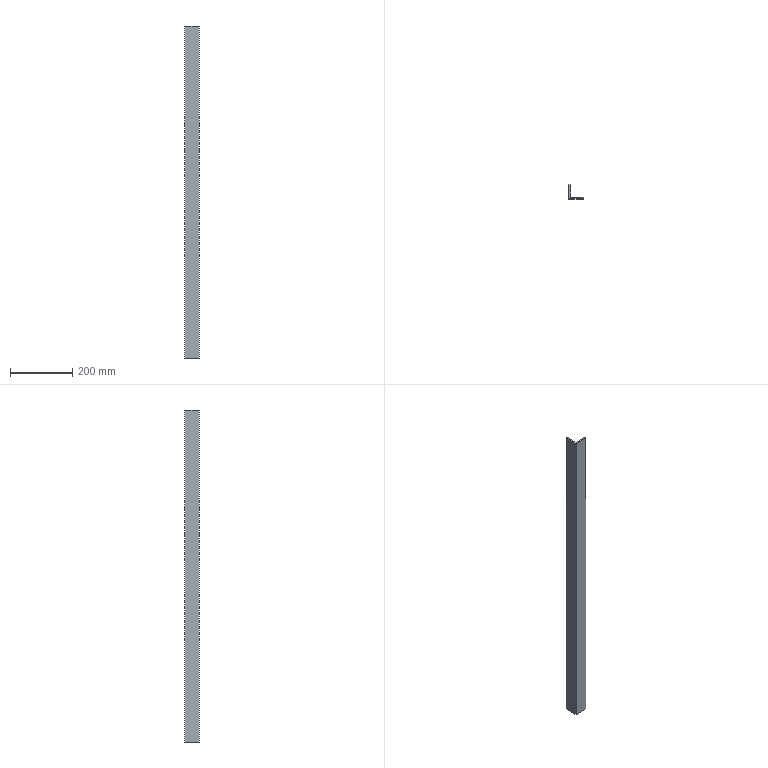Part | SolidWorks | features Extrusion 1 | 1 solid | 8 faces | box 45 x 45 x 1067 mm | volume 453390 mm3 | plane 8
STEP:
#1=CARTESIAN_POINT('',(-19.65,21.953,0.));
#2=VERTEX_POINT('',#1);
#3=CARTESIAN_POINT('',(-24.65,21.953,0.));
#4=VERTEX_POINT('',#3);
#5=CARTESIAN_POINT('',(-19.65,21.953,0.));
#6=DIRECTION('',(-1.,0.,0.));
#7=VECTOR('',#6,1000.);
#8=LINE('',#5,#7);
#9=EDGE_CURVE('',#2,#4,#8,.T.);
#10=ORIENTED_EDGE('',*,*,#9,.T.);
#11=CARTESIAN_POINT('',(-24.65,21.953,1066.8));
#12=VERTEX_POINT('',#11);
#13=CARTESIAN_POINT('',(-24.65,21.953,1066.8));
#14=DIRECTION('',(0.,0.,-1.));
#15=VECTOR('',#14,1000.);
#16=LINE('',#13,#15);
#17=EDGE_CURVE('',#12,#4,#16,.T.);
#18=ORIENTED_EDGE('',*,*,#17,.F.);
#19=CARTESIAN_POINT('',(-19.65,21.953,1066.8));
#20=VERTEX_POINT('',#19);
#21=CARTESIAN_POINT('',(-19.65,21.953,1066.8));
#22=DIRECTION('',(-1.,0.,0.));
#23=VECTOR('',#22,1000.);
#24=LINE('',#21,#23);
#25=EDGE_CURVE('',#20,#12,#24,.T.);
#26=ORIENTED_EDGE('',*,*,#25,.F.);
#27=CARTESIAN_POINT('',(-19.65,21.953,1066.8));
#28=DIRECTION('',(0.,0.,-1.));
#29=VECTOR('',#28,1000.);
#30=LINE('',#27,#29);
#31=EDGE_CURVE('',#20,#2,#30,.T.);
#32=ORIENTED_EDGE('',*,*,#31,.T.);
#33=EDGE_LOOP('',(#10,#18,#26,#32));
#34=FACE_OUTER_BOUND('',#33,.T.);
#35=CARTESIAN_POINT('',(-19.65,21.953,1066.8));
#36=DIRECTION('',(0.,-1.,0.));
#37=DIRECTION('',(1.,0.,0.));
#38=AXIS2_PLACEMENT_3D('',#35,#36,#37);
#39=PLANE('',#38);
#40=ADVANCED_FACE('',(#34),#39,.F.);
#41=CARTESIAN_POINT('',(-24.65,-23.047,0.));
#42=VERTEX_POINT('',#41);
#43=CARTESIAN_POINT('',(-24.65,21.953,0.));
#44=DIRECTION('',(0.,-1.,0.));
#45=VECTOR('',#44,1000.);
#46=LINE('',#43,#45);
#47=EDGE_CURVE('',#4,#42,#46,.T.);
#48=ORIENTED_EDGE('',*,*,#47,.T.);
#49=CARTESIAN_POINT('',(-24.65,-23.047,1066.8));
#50=VERTEX_POINT('',#49);
#51=CARTESIAN_POINT('',(-24.65,-23.047,1066.8));
#52=DIRECTION('',(0.,0.,-1.));
#53=VECTOR('',#52,1000.);
#54=LINE('',#51,#53);
#55=EDGE_CURVE('',#50,#42,#54,.T.);
#56=ORIENTED_EDGE('',*,*,#55,.F.);
#57=CARTESIAN_POINT('',(-24.65,21.953,1066.8));
#58=DIRECTION('',(0.,-1.,0.));
#59=VECTOR('',#58,1000.);
#60=LINE('',#57,#59);
#61=EDGE_CURVE('',#12,#50,#60,.T.);
#62=ORIENTED_EDGE('',*,*,#61,.F.);
#63=ORIENTED_EDGE('',*,*,#17,.T.);
#64=EDGE_LOOP('',(#48,#56,#62,#63));
#65=FACE_OUTER_BOUND('',#64,.T.);
#66=CARTESIAN_POINT('',(-24.65,21.953,1066.8));
#67=DIRECTION('',(1.,0.,0.));
#68=DIRECTION('',(0.,1.,0.));
#69=AXIS2_PLACEMENT_3D('',#66,#67,#68);
#70=PLANE('',#69);
#71=ADVANCED_FACE('',(#65),#70,.F.);
#72=CARTESIAN_POINT('',(20.35,-23.047,0.));
#73=VERTEX_POINT('',#72);
#74=CARTESIAN_POINT('',(-24.65,-23.047,0.));
#75=DIRECTION('',(1.,0.,0.));
#76=VECTOR('',#75,1000.);
#77=LINE('',#74,#76);
#78=EDGE_CURVE('',#42,#73,#77,.T.);
#79=ORIENTED_EDGE('',*,*,#78,.T.);
#80=CARTESIAN_POINT('',(20.35,-23.047,1066.8));
#81=VERTEX_POINT('',#80);
#82=CARTESIAN_POINT('',(20.35,-23.047,1066.8));
#83=DIRECTION('',(0.,0.,-1.));
#84=VECTOR('',#83,1000.);
#85=LINE('',#82,#84);
#86=EDGE_CURVE('',#81,#73,#85,.T.);
#87=ORIENTED_EDGE('',*,*,#86,.F.);
#88=CARTESIAN_POINT('',(-24.65,-23.047,1066.8));
#89=DIRECTION('',(1.,0.,0.));
#90=VECTOR('',#89,1000.);
#91=LINE('',#88,#90);
#92=EDGE_CURVE('',#50,#81,#91,.T.);
#93=ORIENTED_EDGE('',*,*,#92,.F.);
#94=ORIENTED_EDGE('',*,*,#55,.T.);
#95=EDGE_LOOP('',(#79,#87,#93,#94));
#96=FACE_OUTER_BOUND('',#95,.T.);
#97=CARTESIAN_POINT('',(-24.65,-23.047,1066.8));
#98=DIRECTION('',(0.,1.,0.));
#99=DIRECTION('',(0.,0.,1.));
#100=AXIS2_PLACEMENT_3D('',#97,#98,#99);
#101=PLANE('',#100);
#102=ADVANCED_FACE('',(#96),#101,.F.);
#103=CARTESIAN_POINT('',(20.35,-18.047,0.));
#104=VERTEX_POINT('',#103);
#105=CARTESIAN_POINT('',(20.35,-23.047,0.));
#106=DIRECTION('',(0.,1.,0.));
#107=VECTOR('',#106,1000.);
#108=LINE('',#105,#107);
#109=EDGE_CURVE('',#73,#104,#108,.T.);
#110=ORIENTED_EDGE('',*,*,#109,.T.);
#111=CARTESIAN_POINT('',(20.35,-18.047,1066.8));
#112=VERTEX_POINT('',#111);
#113=CARTESIAN_POINT('',(20.35,-18.047,1066.8));
#114=DIRECTION('',(0.,0.,-1.));
#115=VECTOR('',#114,1000.);
#116=LINE('',#113,#115);
#117=EDGE_CURVE('',#112,#104,#116,.T.);
#118=ORIENTED_EDGE('',*,*,#117,.F.);
#119=CARTESIAN_POINT('',(20.35,-23.047,1066.8));
#120=DIRECTION('',(0.,1.,0.));
#121=VECTOR('',#120,1000.);
#122=LINE('',#119,#121);
#123=EDGE_CURVE('',#81,#112,#122,.T.);
#124=ORIENTED_EDGE('',*,*,#123,.F.);
#125=ORIENTED_EDGE('',*,*,#86,.T.);
#126=EDGE_LOOP('',(#110,#118,#124,#125));
#127=FACE_OUTER_BOUND('',#126,.T.);
#128=CARTESIAN_POINT('',(20.35,-23.047,1066.8));
#129=DIRECTION('',(-1.,0.,0.));
#130=DIRECTION('',(0.,0.,1.));
#131=AXIS2_PLACEMENT_3D('',#128,#129,#130);
#132=PLANE('',#131);
#133=ADVANCED_FACE('',(#127),#132,.F.);
#134=CARTESIAN_POINT('',(-19.65,-18.047,0.));
#135=VERTEX_POINT('',#134);
#136=CARTESIAN_POINT('',(20.35,-18.047,0.));
#137=DIRECTION('',(-1.,0.,0.));
#138=VECTOR('',#137,1000.);
#139=LINE('',#136,#138);
#140=EDGE_CURVE('',#104,#135,#139,.T.);
#141=ORIENTED_EDGE('',*,*,#140,.T.);
#142=CARTESIAN_POINT('',(-19.65,-18.047,1066.8));
#143=VERTEX_POINT('',#142);
#144=CARTESIAN_POINT('',(-19.65,-18.047,1066.8));
#145=DIRECTION('',(0.,0.,-1.));
#146=VECTOR('',#145,1000.);
#147=LINE('',#144,#146);
#148=EDGE_CURVE('',#143,#135,#147,.T.);
#149=ORIENTED_EDGE('',*,*,#148,.F.);
#150=CARTESIAN_POINT('',(20.35,-18.047,1066.8));
#151=DIRECTION('',(-1.,0.,0.));
#152=VECTOR('',#151,1000.);
#153=LINE('',#150,#152);
#154=EDGE_CURVE('',#112,#143,#153,.T.);
#155=ORIENTED_EDGE('',*,*,#154,.F.);
#156=ORIENTED_EDGE('',*,*,#117,.T.);
#157=EDGE_LOOP('',(#141,#149,#155,#156));
#158=FACE_OUTER_BOUND('',#157,.T.);
#159=CARTESIAN_POINT('',(20.35,-18.047,1066.8));
#160=DIRECTION('',(0.,-1.,0.));
#161=DIRECTION('',(1.,0.,0.));
#162=AXIS2_PLACEMENT_3D('',#159,#160,#161);
#163=PLANE('',#162);
#164=ADVANCED_FACE('',(#158),#163,.F.);
#165=CARTESIAN_POINT('',(-19.65,-18.047,0.));
#166=DIRECTION('',(0.,1.,0.));
#167=VECTOR('',#166,1000.);
#168=LINE('',#165,#167);
#169=EDGE_CURVE('',#135,#2,#168,.T.);
#170=ORIENTED_EDGE('',*,*,#169,.T.);
#171=ORIENTED_EDGE('',*,*,#31,.F.);
#172=CARTESIAN_POINT('',(-19.65,-18.047,1066.8));
#173=DIRECTION('',(0.,1.,0.));
#174=VECTOR('',#173,1000.);
#175=LINE('',#172,#174);
#176=EDGE_CURVE('',#143,#20,#175,.T.);
#177=ORIENTED_EDGE('',*,*,#176,.F.);
#178=ORIENTED_EDGE('',*,*,#148,.T.);
#179=EDGE_LOOP('',(#170,#171,#177,#178));
#180=FACE_OUTER_BOUND('',#179,.T.);
#181=CARTESIAN_POINT('',(-19.65,-18.047,1066.8));
#182=DIRECTION('',(-1.,0.,0.));
#183=DIRECTION('',(0.,-1.,0.));
#184=AXIS2_PLACEMENT_3D('',#181,#182,#183);
#185=PLANE('',#184);
#186=ADVANCED_FACE('',(#180),#185,.F.);
#187=ORIENTED_EDGE('',*,*,#25,.T.);
#188=ORIENTED_EDGE('',*,*,#61,.T.);
#189=ORIENTED_EDGE('',*,*,#92,.T.);
#190=ORIENTED_EDGE('',*,*,#123,.T.);
#191=ORIENTED_EDGE('',*,*,#154,.T.);
#192=ORIENTED_EDGE('',*,*,#176,.T.);
#193=EDGE_LOOP('',(#187,#188,#189,#190,#191,#192));
#194=FACE_OUTER_BOUND('',#193,.T.);
#195=CARTESIAN_POINT('',(-24.65,21.953,1066.8));
#196=DIRECTION('',(0.,0.,1.));
#197=DIRECTION('',(1.,0.,0.));
#198=AXIS2_PLACEMENT_3D('',#195,#196,#197);
#199=PLANE('',#198);
#200=ADVANCED_FACE('',(#194),#199,.T.);
#201=ORIENTED_EDGE('',*,*,#9,.F.);
#202=ORIENTED_EDGE('',*,*,#169,.F.);
#203=ORIENTED_EDGE('',*,*,#140,.F.);
#204=ORIENTED_EDGE('',*,*,#109,.F.);
#205=ORIENTED_EDGE('',*,*,#78,.F.);
#206=ORIENTED_EDGE('',*,*,#47,.F.);
#207=EDGE_LOOP('',(#201,#202,#203,#204,#205,#206));
#208=FACE_OUTER_BOUND('',#207,.T.);
#209=CARTESIAN_POINT('',(-24.65,21.953,0.));
#210=DIRECTION('',(0.,0.,1.));
#211=DIRECTION('',(1.,0.,0.));
#212=AXIS2_PLACEMENT_3D('',#209,#210,#211);
#213=PLANE('',#212);
#214=ADVANCED_FACE('',(#208),#213,.F.);
#215=CLOSED_SHELL('',(#40,#71,#102,#133,#164,#186,#200,#214));
#216=MANIFOLD_SOLID_BREP('',#215);
#217=CARTESIAN_POINT('',(0.,0.,0.));
#218=DIRECTION('',(0.,0.,1.));
#219=DIRECTION('',(1.,0.,0.));
#220=AXIS2_PLACEMENT_3D('',#217,#218,#219);
#221=(LENGTH_UNIT()NAMED_UNIT(*)SI_UNIT(.MILLI.,.METRE.));
#222=UNCERTAINTY_MEASURE_WITH_UNIT(LENGTH_MEASURE(0.00001),#221,'','');
#223=(NAMED_UNIT(*)PLANE_ANGLE_UNIT()SI_UNIT($,.RADIAN.));
#224=(NAMED_UNIT(*)SI_UNIT($,.STERADIAN.)SOLID_ANGLE_UNIT());
#225=(GEOMETRIC_REPRESENTATION_CONTEXT(3)GLOBAL_UNCERTAINTY_ASSIGNED_CONTEXT((#222))GLOBAL_UNIT_ASSIGNED_CONTEXT((#221,#223,#224))REPRESENTATION_CONTEXT('',''));
#226=ADVANCED_BREP_SHAPE_REPRESENTATION('',(#216,#220),#225);